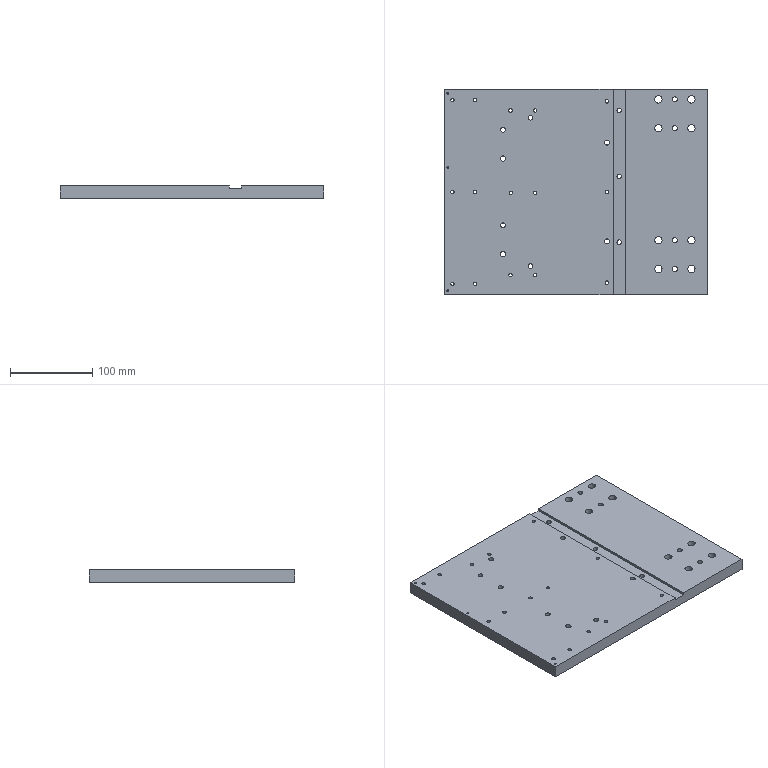CAM job | NX | 3-axis milling, drilling | part box 320 x 250 x 15 mm | stock box 326 x 256 x 16 mm
Tools:
number,name,description,diameter,corner_radius,flute_length,length,flutes
7,D6A45,Milling Tool-5 Parameters,6.0,0.0,3.0,3.0,2
10,D10,Milling Tool-5 Parameters,10.0,0.0,50.0,75.0,2
11,D10JING,Milling Tool-5 Parameters,10.0,0.0,50.0,75.0,2
8,2.5ZT,Drilling Tool,2.5,0.0,35.0,50.0,2
9,M3,Milling Tool-5 Parameters,2.5,0.0,30.0,30.0,4
14,4.2ZT,Drilling Tool,4.2,0.0,35.0,50.0,2
15,M5,Milling Tool-5 Parameters,4.2,0.0,30.0,30.0,4
18,5.8ZT,Drilling Tool,5.8,0.0,35.0,50.0,2
20,6.0JD,Milling Tool-5 Parameters,6.0,0.0,30.0,30.0,4
12,5.5ZT,Drilling Tool,5.5,0.0,35.0,50.0,2
19,9.0ZT,Drilling Tool,9.0,0.0,35.0,50.0,2
4,D4,Milling Tool-5 Parameters,4.0,0.0,50.0,75.0,2
Operations:
program,operation,operation_type,tool,method,geometry_group,spindle_rpm,surface_speed,feed_per_tooth,feed_cut,feed_plunge,cut_length_mm,path_length_mm,cut_time_min,machine_time_min
1-323-253-15毛胚-AB胶,FLOOR_WALL,VolumeBased25DMillingOperation,D10JING,METHOD,A,6500.0,1286.0,0.0962,1250.0,100.0,14711.997,14765.997,11.77,11.775
1-323-253-15毛胚-AB胶,DRILLING_COPY_1,Operation,D6A45,METHOD,A,3000.0,56.0,0.0333,200.0,0.0,164.0,1887.564,0.82,0.9924
1-323-253-15毛胚-AB胶,DRILLING_COPY_1_COPY_1,Operation,2.5ZT,METHOD,A,2000.0,15.0,0.0375,150.0,0.0,60.753,427.586,0.405,0.4417
1-323-253-15毛胚-AB胶,DRILLING_COPY_1_COPY_COPY_2,Operation,M3,METHOD,A,200.0,1.0,0.125,100.0,0.0,55.5,417.08,0.555,0.5912
1-323-253-15毛胚-AB胶,DRILLING_COPY_1_COPY,Operation,4.2ZT,METHOD,A,2000.0,15.0,0.0375,150.0,0.0,311.427,1514.553,2.076,2.196
1-323-253-15毛胚-AB胶,DRILLING_COPY_1_COPY_COPY,Operation,M5,METHOD,A,200.0,2.0,0.2,160.0,0.0,277.5,1446.699,1.734,1.851
1-323-253-15毛胚-AB胶,DRILLING_COPY_1_COPY_COPY_1,Operation,5.8ZT,METHOD,A,2000.0,18.0,0.03,120.0,0.0,254.91,1259.194,2.124,2.225
1-323-253-15毛胚-AB胶,DRILLING_COPY_1_COPY_COPY_1_COPY,Operation,6.0JD,METHOD,A,1000.0,9.0,0.01,40.0,0.0,185.0,1101.541,4.625,4.717
1-323-253-15毛胚-AB胶,DRILLING_COPY_1_COPY_COPY_1_COPY_1,Operation,5.5ZT,METHOD,A,2000.0,18.0,0.03,120.0,0.0,58.957,344.027,0.4913,0.5198
1-323-253-15毛胚-AB胶,DRILLING_COPY_1_COPY_COPY_1_COPY_1_COPY,Operation,9.0ZT,METHOD,A,2000.0,18.0,0.03,120.0,0.0,165.631,769.002,1.38,1.441
1-323-253-15毛胚-AB胶,ZLEVEL_PROFILE,ZLevelMilling,D10,METHOD,A,7000.0,219.0,0.2143,3000.0,1000.0,17684.283,17755.683,5.926,5.933
1-323-253-15毛胚-AB胶,刀补11_COPY,VolumeBased25DMillingOperation,D10,METHOD,A,7000.0,219.0,0.1429,2000.0,100.0,1599.895,1676.495,0.7999,0.8078
1-323-253-15毛胚-AB胶,ZLEVEL_PROFILE_COPY,ZLevelMilling,D4,METHOD,A,7000.0,87.0,0.0857,1200.0,1000.0,745.019,1006.428,0.6323,0.6585
1-323-253-15毛胚-AB胶,ZLEVEL_PROFILE_COPY_1_COPY_COPY_COPY_COPY_2_COPY,ZLevelMilling,D6A45,METHOD,A,7000.0,131.0,0.0714,1000.0,1000.0,2175.284,9266.142,2.175,2.884
1-323-253-15毛胚-AB胶,刀补11,VolumeBased25DMillingOperation,D10JING,METHOD,A,7000.0,87.0,0.0714,1000.0,100.0,533.61,596.61,0.5336,0.5399
1-323-253-15毛胚-AB胶,刀补4,ZLevelMilling,D4,METHOD,A,7000.0,87.0,0.0607,850.0,1000.0,225.226,493.825,0.2646,0.2915
1-323-253-15毛胚-AB胶,ZLEVEL_PROFILE_COPY_1,ZLevelMilling,D10JING,METHOD,A,7000.0,219.0,0.0714,1000.0,1000.0,3556.418,3643.168,3.556,3.565